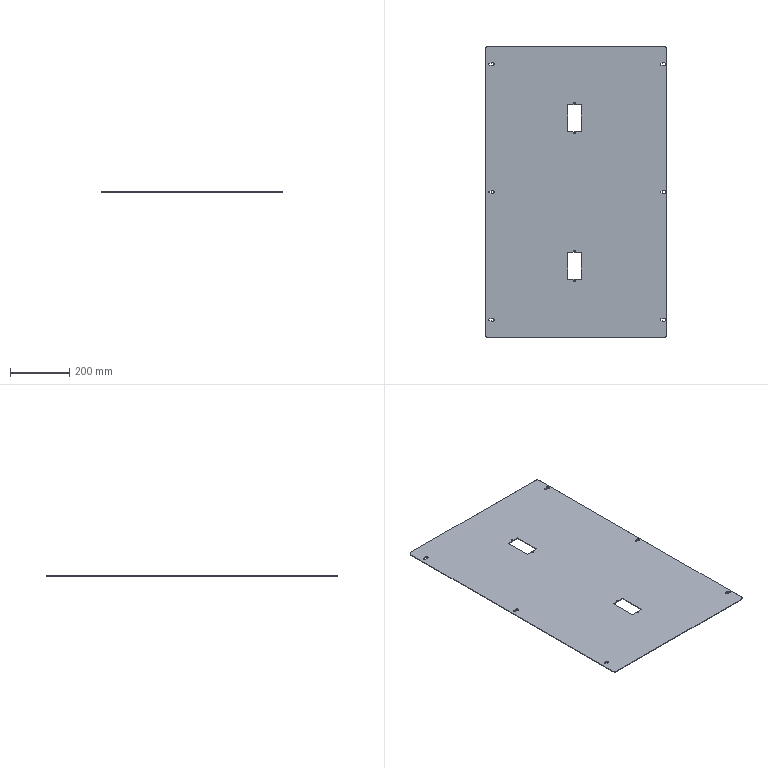Part | SolidWorks | features ICE 4, Extrusion 1, Fillet 1, LPattern 1 | 1 solid | 56 faces | box 615 x 985 x 2 mm | volume 1193141 mm3 | cylinder 30 | plane 26 | commonest cylinder face diameters 6.6 x12 4.5 x8 11 x6 20 x4